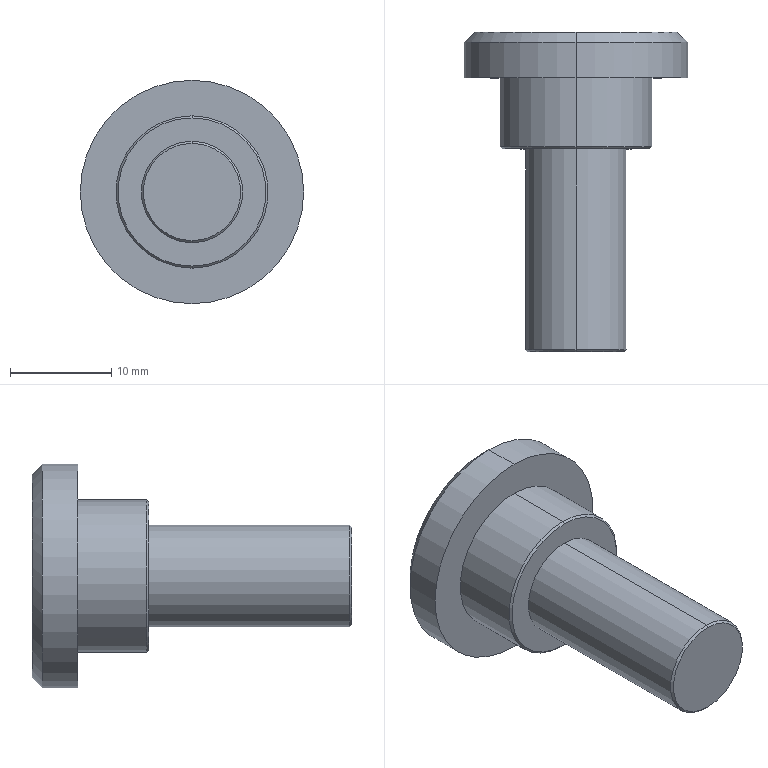Part | SolidWorks | features Chamfer 3, ICE 3, Extrusion 1 | 1 solid | 23 faces | box 22 x 31.5 x 22 mm | volume 4428 mm3 | plane 11 | cone 6 | cylinder 6 | commonest cylinder face diameters 10 x2 15 x2 22 x2
STEP:
#1=CARTESIAN_POINT('',(0.,0.,-4.8));
#2=VERTEX_POINT('',#1);
#3=CARTESIAN_POINT('',(0.,0.,4.8));
#4=VERTEX_POINT('',#3);
#5=CARTESIAN_POINT('',(0.,0.,0.));
#6=DIRECTION('',(0.,-1.,0.));
#7=DIRECTION('',(0.,0.,1.));
#8=AXIS2_PLACEMENT_3D('',#5,#6,#7);
#9=CIRCLE('',#8,4.8);
#10=EDGE_CURVE('',#2,#4,#9,.T.);
#11=ORIENTED_EDGE('',*,*,#10,.F.);
#12=CARTESIAN_POINT('',(0.,0.2,-5.));
#13=VERTEX_POINT('',#12);
#14=CARTESIAN_POINT('',(0.,0.2,-5.));
#15=DIRECTION('',(0.,0.7071,-0.7071));
#16=VECTOR('',#15,1000.);
#17=LINE('',#14,#16);
#18=EDGE_CURVE('',#2,#13,#17,.T.);
#19=ORIENTED_EDGE('',*,*,#18,.T.);
#20=CARTESIAN_POINT('',(0.,0.2,5.));
#21=VERTEX_POINT('',#20);
#22=CARTESIAN_POINT('',(0.,0.2,0.));
#23=DIRECTION('',(0.,1.,0.));
#24=DIRECTION('',(0.,0.,1.));
#25=AXIS2_PLACEMENT_3D('',#22,#23,#24);
#26=CIRCLE('',#25,5.);
#27=EDGE_CURVE('',#21,#13,#26,.T.);
#28=ORIENTED_EDGE('',*,*,#27,.F.);
#29=CARTESIAN_POINT('',(0.,0.2,5.));
#30=DIRECTION('',(0.,0.7071,0.7071));
#31=VECTOR('',#30,1000.);
#32=LINE('',#29,#31);
#33=EDGE_CURVE('',#4,#21,#32,.T.);
#34=ORIENTED_EDGE('',*,*,#33,.F.);
#35=EDGE_LOOP('',(#11,#19,#28,#34));
#36=FACE_OUTER_BOUND('',#35,.T.);
#37=CARTESIAN_POINT('',(0.,0.2,0.));
#38=DIRECTION('',(0.,1.,0.));
#39=DIRECTION('',(0.,0.,1.));
#40=AXIS2_PLACEMENT_3D('',#37,#38,#39);
#41=CONICAL_SURFACE('',#40,5.,0.7854);
#42=ADVANCED_FACE('',(#36),#41,.T.);
#43=CARTESIAN_POINT('',(0.,20.,-7.3));
#44=VERTEX_POINT('',#43);
#45=CARTESIAN_POINT('',(0.,20.,7.3));
#46=VERTEX_POINT('',#45);
#47=CARTESIAN_POINT('',(0.,20.,0.));
#48=DIRECTION('',(0.,-1.,0.));
#49=DIRECTION('',(0.,0.,1.));
#50=AXIS2_PLACEMENT_3D('',#47,#48,#49);
#51=CIRCLE('',#50,7.3);
#52=EDGE_CURVE('',#44,#46,#51,.T.);
#53=ORIENTED_EDGE('',*,*,#52,.F.);
#54=CARTESIAN_POINT('',(0.,20.2,-7.5));
#55=VERTEX_POINT('',#54);
#56=CARTESIAN_POINT('',(0.,20.2,-7.5));
#57=DIRECTION('',(0.,0.7071,-0.7071));
#58=VECTOR('',#57,1000.);
#59=LINE('',#56,#58);
#60=EDGE_CURVE('',#44,#55,#59,.T.);
#61=ORIENTED_EDGE('',*,*,#60,.T.);
#62=CARTESIAN_POINT('',(0.,20.2,7.5));
#63=VERTEX_POINT('',#62);
#64=CARTESIAN_POINT('',(0.,20.2,0.));
#65=DIRECTION('',(0.,1.,0.));
#66=DIRECTION('',(0.,0.,1.));
#67=AXIS2_PLACEMENT_3D('',#64,#65,#66);
#68=CIRCLE('',#67,7.5);
#69=EDGE_CURVE('',#63,#55,#68,.T.);
#70=ORIENTED_EDGE('',*,*,#69,.F.);
#71=CARTESIAN_POINT('',(0.,20.2,7.5));
#72=DIRECTION('',(0.,0.7071,0.7071));
#73=VECTOR('',#72,1000.);
#74=LINE('',#71,#73);
#75=EDGE_CURVE('',#46,#63,#74,.T.);
#76=ORIENTED_EDGE('',*,*,#75,.F.);
#77=EDGE_LOOP('',(#53,#61,#70,#76));
#78=FACE_OUTER_BOUND('',#77,.T.);
#79=CARTESIAN_POINT('',(0.,20.2,0.));
#80=DIRECTION('',(0.,1.,0.));
#81=DIRECTION('',(0.,0.,1.));
#82=AXIS2_PLACEMENT_3D('',#79,#80,#81);
#83=CONICAL_SURFACE('',#82,7.5,0.7854);
#84=ADVANCED_FACE('',(#78),#83,.T.);
#85=CARTESIAN_POINT('',(0.,31.5,10.));
#86=VERTEX_POINT('',#85);
#87=CARTESIAN_POINT('',(0.,31.5,-10.));
#88=VERTEX_POINT('',#87);
#89=CARTESIAN_POINT('',(0.,31.5,0.));
#90=DIRECTION('',(0.,1.,0.));
#91=DIRECTION('',(0.,0.,1.));
#92=AXIS2_PLACEMENT_3D('',#89,#90,#91);
#93=CIRCLE('',#92,10.);
#94=EDGE_CURVE('',#86,#88,#93,.T.);
#95=ORIENTED_EDGE('',*,*,#94,.F.);
#96=CARTESIAN_POINT('',(0.,30.5,11.));
#97=VERTEX_POINT('',#96);
#98=CARTESIAN_POINT('',(0.,31.5,10.));
#99=DIRECTION('',(0.,-0.7071,0.7071));
#100=VECTOR('',#99,1000.);
#101=LINE('',#98,#100);
#102=EDGE_CURVE('',#86,#97,#101,.T.);
#103=ORIENTED_EDGE('',*,*,#102,.T.);
#104=CARTESIAN_POINT('',(0.,30.5,-11.));
#105=VERTEX_POINT('',#104);
#106=CARTESIAN_POINT('',(0.,30.5,0.));
#107=DIRECTION('',(0.,-1.,0.));
#108=DIRECTION('',(0.,0.,1.));
#109=AXIS2_PLACEMENT_3D('',#106,#107,#108);
#110=CIRCLE('',#109,11.);
#111=EDGE_CURVE('',#105,#97,#110,.T.);
#112=ORIENTED_EDGE('',*,*,#111,.F.);
#113=CARTESIAN_POINT('',(0.,31.5,-10.));
#114=DIRECTION('',(0.,-0.7071,-0.7071));
#115=VECTOR('',#114,1000.);
#116=LINE('',#113,#115);
#117=EDGE_CURVE('',#88,#105,#116,.T.);
#118=ORIENTED_EDGE('',*,*,#117,.F.);
#119=EDGE_LOOP('',(#95,#103,#112,#118));
#120=FACE_OUTER_BOUND('',#119,.T.);
#121=CARTESIAN_POINT('',(0.,31.5,0.));
#122=DIRECTION('',(0.,-1.,0.));
#123=DIRECTION('',(0.,0.,-1.));
#124=AXIS2_PLACEMENT_3D('',#121,#122,#123);
#125=CONICAL_SURFACE('',#124,10.,0.7854);
#126=ADVANCED_FACE('',(#120),#125,.T.);
#127=ORIENTED_EDGE('',*,*,#111,.T.);
#128=CARTESIAN_POINT('',(0.,27.,11.));
#129=VERTEX_POINT('',#128);
#130=CARTESIAN_POINT('',(0.,31.5,11.));
#131=DIRECTION('',(0.,-1.,0.));
#132=VECTOR('',#131,1000.);
#133=LINE('',#130,#132);
#134=EDGE_CURVE('',#97,#129,#133,.T.);
#135=ORIENTED_EDGE('',*,*,#134,.T.);
#136=CARTESIAN_POINT('',(0.,27.,-11.));
#137=VERTEX_POINT('',#136);
#138=CARTESIAN_POINT('',(0.,27.,0.));
#139=DIRECTION('',(0.,1.,0.));
#140=DIRECTION('',(0.,0.,1.));
#141=AXIS2_PLACEMENT_3D('',#138,#139,#140);
#142=CIRCLE('',#141,11.);
#143=EDGE_CURVE('',#129,#137,#142,.T.);
#144=ORIENTED_EDGE('',*,*,#143,.T.);
#145=CARTESIAN_POINT('',(0.,31.5,-11.));
#146=DIRECTION('',(0.,-1.,0.));
#147=VECTOR('',#146,1000.);
#148=LINE('',#145,#147);
#149=EDGE_CURVE('',#105,#137,#148,.T.);
#150=ORIENTED_EDGE('',*,*,#149,.F.);
#151=EDGE_LOOP('',(#127,#135,#144,#150));
#152=FACE_OUTER_BOUND('',#151,.T.);
#153=CARTESIAN_POINT('',(0.,31.5,0.));
#154=DIRECTION('',(0.,-1.,0.));
#155=DIRECTION('',(0.,0.,-1.));
#156=AXIS2_PLACEMENT_3D('',#153,#154,#155);
#157=CYLINDRICAL_SURFACE('',#156,11.);
#158=ADVANCED_FACE('',(#152),#157,.T.);
#159=CARTESIAN_POINT('',(0.,27.,7.5));
#160=VERTEX_POINT('',#159);
#161=CARTESIAN_POINT('',(0.,27.,-7.5));
#162=VERTEX_POINT('',#161);
#163=CARTESIAN_POINT('',(0.,27.,0.));
#164=DIRECTION('',(0.,1.,0.));
#165=DIRECTION('',(0.,0.,1.));
#166=AXIS2_PLACEMENT_3D('',#163,#164,#165);
#167=CIRCLE('',#166,7.5);
#168=EDGE_CURVE('',#160,#162,#167,.T.);
#169=ORIENTED_EDGE('',*,*,#168,.F.);
#170=CARTESIAN_POINT('',(0.,27.,7.5));
#171=DIRECTION('',(0.,-1.,0.));
#172=VECTOR('',#171,1000.);
#173=LINE('',#170,#172);
#174=EDGE_CURVE('',#160,#63,#173,.T.);
#175=ORIENTED_EDGE('',*,*,#174,.T.);
#176=ORIENTED_EDGE('',*,*,#69,.T.);
#177=CARTESIAN_POINT('',(0.,27.,-7.5));
#178=DIRECTION('',(0.,-1.,0.));
#179=VECTOR('',#178,1000.);
#180=LINE('',#177,#179);
#181=EDGE_CURVE('',#162,#55,#180,.T.);
#182=ORIENTED_EDGE('',*,*,#181,.F.);
#183=EDGE_LOOP('',(#169,#175,#176,#182));
#184=FACE_OUTER_BOUND('',#183,.T.);
#185=CARTESIAN_POINT('',(0.,27.,0.));
#186=DIRECTION('',(0.,-1.,0.));
#187=DIRECTION('',(0.,0.,-1.));
#188=AXIS2_PLACEMENT_3D('',#185,#186,#187);
#189=CYLINDRICAL_SURFACE('',#188,7.5);
#190=ADVANCED_FACE('',(#184),#189,.T.);
#191=CARTESIAN_POINT('',(0.,20.,5.));
#192=VERTEX_POINT('',#191);
#193=CARTESIAN_POINT('',(0.,20.,-5.));
#194=VERTEX_POINT('',#193);
#195=CARTESIAN_POINT('',(0.,20.,0.));
#196=DIRECTION('',(0.,1.,0.));
#197=DIRECTION('',(0.,0.,1.));
#198=AXIS2_PLACEMENT_3D('',#195,#196,#197);
#199=CIRCLE('',#198,5.);
#200=EDGE_CURVE('',#192,#194,#199,.T.);
#201=ORIENTED_EDGE('',*,*,#200,.F.);
#202=CARTESIAN_POINT('',(0.,20.,5.));
#203=DIRECTION('',(0.,-1.,0.));
#204=VECTOR('',#203,1000.);
#205=LINE('',#202,#204);
#206=EDGE_CURVE('',#192,#21,#205,.T.);
#207=ORIENTED_EDGE('',*,*,#206,.T.);
#208=ORIENTED_EDGE('',*,*,#27,.T.);
#209=CARTESIAN_POINT('',(0.,20.,-5.));
#210=DIRECTION('',(0.,-1.,0.));
#211=VECTOR('',#210,1000.);
#212=LINE('',#209,#211);
#213=EDGE_CURVE('',#194,#13,#212,.T.);
#214=ORIENTED_EDGE('',*,*,#213,.F.);
#215=EDGE_LOOP('',(#201,#207,#208,#214));
#216=FACE_OUTER_BOUND('',#215,.T.);
#217=CARTESIAN_POINT('',(0.,20.,0.));
#218=DIRECTION('',(0.,-1.,0.));
#219=DIRECTION('',(0.,0.,-1.));
#220=AXIS2_PLACEMENT_3D('',#217,#218,#219);
#221=CYLINDRICAL_SURFACE('',#220,5.);
#222=ADVANCED_FACE('',(#216),#221,.T.);
#223=ORIENTED_EDGE('',*,*,#206,.F.);
#224=CARTESIAN_POINT('',(0.,20.,0.));
#225=DIRECTION('',(0.,1.,0.));
#226=DIRECTION('',(0.,0.,1.));
#227=AXIS2_PLACEMENT_3D('',#224,#225,#226);
#228=CIRCLE('',#227,5.);
#229=EDGE_CURVE('',#194,#192,#228,.T.);
#230=ORIENTED_EDGE('',*,*,#229,.F.);
#231=ORIENTED_EDGE('',*,*,#213,.T.);
#232=CARTESIAN_POINT('',(0.,0.2,0.));
#233=DIRECTION('',(0.,1.,0.));
#234=DIRECTION('',(0.,0.,1.));
#235=AXIS2_PLACEMENT_3D('',#232,#233,#234);
#236=CIRCLE('',#235,5.);
#237=EDGE_CURVE('',#13,#21,#236,.T.);
#238=ORIENTED_EDGE('',*,*,#237,.T.);
#239=EDGE_LOOP('',(#223,#230,#231,#238));
#240=FACE_OUTER_BOUND('',#239,.T.);
#241=CARTESIAN_POINT('',(0.,20.,0.));
#242=DIRECTION('',(0.,-1.,0.));
#243=DIRECTION('',(0.,0.,-1.));
#244=AXIS2_PLACEMENT_3D('',#241,#242,#243);
#245=CYLINDRICAL_SURFACE('',#244,5.);
#246=ADVANCED_FACE('',(#240),#245,.T.);
#247=CARTESIAN_POINT('',(0.,0.,0.));
#248=DIRECTION('',(0.,-1.,0.));
#249=DIRECTION('',(0.,0.,1.));
#250=AXIS2_PLACEMENT_3D('',#247,#248,#249);
#251=CIRCLE('',#250,4.8);
#252=EDGE_CURVE('',#4,#2,#251,.T.);
#253=ORIENTED_EDGE('',*,*,#252,.T.);
#254=ORIENTED_EDGE('',*,*,#10,.T.);
#255=EDGE_LOOP('',(#253,#254));
#256=FACE_OUTER_BOUND('',#255,.T.);
#257=CARTESIAN_POINT('',(0.,0.,0.));
#258=DIRECTION('',(0.,1.,0.));
#259=DIRECTION('',(0.,0.,1.));
#260=AXIS2_PLACEMENT_3D('',#257,#258,#259);
#261=PLANE('',#260);
#262=ADVANCED_FACE('',(#256),#261,.F.);
#263=CARTESIAN_POINT('',(0.,20.,0.));
#264=DIRECTION('',(0.,-1.,0.));
#265=DIRECTION('',(0.,0.,1.));
#266=AXIS2_PLACEMENT_3D('',#263,#264,#265);
#267=CIRCLE('',#266,7.3);
#268=EDGE_CURVE('',#46,#44,#267,.T.);
#269=ORIENTED_EDGE('',*,*,#268,.T.);
#270=ORIENTED_EDGE('',*,*,#52,.T.);
#271=EDGE_LOOP('',(#269,#270));
#272=FACE_OUTER_BOUND('',#271,.T.);
#273=ORIENTED_EDGE('',*,*,#229,.T.);
#274=ORIENTED_EDGE('',*,*,#200,.T.);
#275=EDGE_LOOP('',(#273,#274));
#276=FACE_BOUND('',#275,.T.);
#277=CARTESIAN_POINT('',(0.,20.,0.));
#278=DIRECTION('',(0.,1.,0.));
#279=DIRECTION('',(0.,0.,1.));
#280=AXIS2_PLACEMENT_3D('',#277,#278,#279);
#281=PLANE('',#280);
#282=ADVANCED_FACE('',(#272,#276),#281,.F.);
#283=ORIENTED_EDGE('',*,*,#174,.F.);
#284=CARTESIAN_POINT('',(0.,27.,0.));
#285=DIRECTION('',(0.,1.,0.));
#286=DIRECTION('',(0.,0.,1.));
#287=AXIS2_PLACEMENT_3D('',#284,#285,#286);
#288=CIRCLE('',#287,7.5);
#289=EDGE_CURVE('',#162,#160,#288,.T.);
#290=ORIENTED_EDGE('',*,*,#289,.F.);
#291=ORIENTED_EDGE('',*,*,#181,.T.);
#292=CARTESIAN_POINT('',(0.,20.2,0.));
#293=DIRECTION('',(0.,1.,0.));
#294=DIRECTION('',(0.,0.,1.));
#295=AXIS2_PLACEMENT_3D('',#292,#293,#294);
#296=CIRCLE('',#295,7.5);
#297=EDGE_CURVE('',#55,#63,#296,.T.);
#298=ORIENTED_EDGE('',*,*,#297,.T.);
#299=EDGE_LOOP('',(#283,#290,#291,#298));
#300=FACE_OUTER_BOUND('',#299,.T.);
#301=CARTESIAN_POINT('',(0.,27.,0.));
#302=DIRECTION('',(0.,-1.,0.));
#303=DIRECTION('',(0.,0.,-1.));
#304=AXIS2_PLACEMENT_3D('',#301,#302,#303);
#305=CYLINDRICAL_SURFACE('',#304,7.5);
#306=ADVANCED_FACE('',(#300),#305,.T.);
#307=CARTESIAN_POINT('',(0.,27.,0.));
#308=DIRECTION('',(0.,1.,0.));
#309=DIRECTION('',(0.,0.,1.));
#310=AXIS2_PLACEMENT_3D('',#307,#308,#309);
#311=CIRCLE('',#310,11.);
#312=EDGE_CURVE('',#137,#129,#311,.T.);
#313=ORIENTED_EDGE('',*,*,#312,.F.);
#314=ORIENTED_EDGE('',*,*,#143,.F.);
#315=EDGE_LOOP('',(#313,#314));
#316=FACE_OUTER_BOUND('',#315,.T.);
#317=ORIENTED_EDGE('',*,*,#289,.T.);
#318=ORIENTED_EDGE('',*,*,#168,.T.);
#319=EDGE_LOOP('',(#317,#318));
#320=FACE_BOUND('',#319,.T.);
#321=CARTESIAN_POINT('',(0.,27.,0.));
#322=DIRECTION('',(0.,1.,0.));
#323=DIRECTION('',(0.,0.,1.));
#324=AXIS2_PLACEMENT_3D('',#321,#322,#323);
#325=PLANE('',#324);
#326=ADVANCED_FACE('',(#316,#320),#325,.F.);
#327=ORIENTED_EDGE('',*,*,#134,.F.);
#328=CARTESIAN_POINT('',(0.,30.5,0.));
#329=DIRECTION('',(0.,-1.,0.));
#330=DIRECTION('',(0.,0.,1.));
#331=AXIS2_PLACEMENT_3D('',#328,#329,#330);
#332=CIRCLE('',#331,11.);
#333=EDGE_CURVE('',#97,#105,#332,.T.);
#334=ORIENTED_EDGE('',*,*,#333,.T.);
#335=ORIENTED_EDGE('',*,*,#149,.T.);
#336=ORIENTED_EDGE('',*,*,#312,.T.);
#337=EDGE_LOOP('',(#327,#334,#335,#336));
#338=FACE_OUTER_BOUND('',#337,.T.);
#339=CARTESIAN_POINT('',(0.,31.5,0.));
#340=DIRECTION('',(0.,-1.,0.));
#341=DIRECTION('',(0.,0.,-1.));
#342=AXIS2_PLACEMENT_3D('',#339,#340,#341);
#343=CYLINDRICAL_SURFACE('',#342,11.);
#344=ADVANCED_FACE('',(#338),#343,.T.);
#345=CARTESIAN_POINT('',(1.155,31.5,2.));
#346=VERTEX_POINT('',#345);
#347=CARTESIAN_POINT('',(2.309,31.5,0.));
#348=VERTEX_POINT('',#347);
#349=CARTESIAN_POINT('',(1.155,31.5,2.));
#350=DIRECTION('',(0.5,0.,-0.866));
#351=VECTOR('',#350,1000.);
#352=LINE('',#349,#351);
#353=EDGE_CURVE('',#346,#348,#352,.T.);
#354=ORIENTED_EDGE('',*,*,#353,.F.);
#355=CARTESIAN_POINT('',(-1.155,31.5,2.));
#356=VERTEX_POINT('',#355);
#357=CARTESIAN_POINT('',(-1.155,31.5,2.));
#358=DIRECTION('',(1.,0.,0.));
#359=VECTOR('',#358,1000.);
#360=LINE('',#357,#359);
#361=EDGE_CURVE('',#356,#346,#360,.T.);
#362=ORIENTED_EDGE('',*,*,#361,.F.);
#363=CARTESIAN_POINT('',(-2.309,31.5,0.));
#364=VERTEX_POINT('',#363);
#365=CARTESIAN_POINT('',(-2.309,31.5,0.));
#366=DIRECTION('',(0.5,0.,0.866));
#367=VECTOR('',#366,1000.);
#368=LINE('',#365,#367);
#369=EDGE_CURVE('',#364,#356,#368,.T.);
#370=ORIENTED_EDGE('',*,*,#369,.F.);
#371=CARTESIAN_POINT('',(-1.155,31.5,-2.));
#372=VERTEX_POINT('',#371);
#373=CARTESIAN_POINT('',(-1.155,31.5,-2.));
#374=DIRECTION('',(-0.5,0.,0.866));
#375=VECTOR('',#374,1000.);
#376=LINE('',#373,#375);
#377=EDGE_CURVE('',#372,#364,#376,.T.);
#378=ORIENTED_EDGE('',*,*,#377,.F.);
#379=CARTESIAN_POINT('',(1.155,31.5,-2.));
#380=VERTEX_POINT('',#379);
#381=CARTESIAN_POINT('',(1.155,31.5,-2.));
#382=DIRECTION('',(-1.,0.,0.));
#383=VECTOR('',#382,1000.);
#384=LINE('',#381,#383);
#385=EDGE_CURVE('',#380,#372,#384,.T.);
#386=ORIENTED_EDGE('',*,*,#385,.F.);
#387=CARTESIAN_POINT('',(2.309,31.5,0.));
#388=DIRECTION('',(-0.5,0.,-0.866));
#389=VECTOR('',#388,1000.);
#390=LINE('',#387,#389);
#391=EDGE_CURVE('',#348,#380,#390,.T.);
#392=ORIENTED_EDGE('',*,*,#391,.F.);
#393=EDGE_LOOP('',(#354,#362,#370,#378,#386,#392));
#394=FACE_BOUND('',#393,.T.);
#395=CARTESIAN_POINT('',(0.,31.5,0.));
#396=DIRECTION('',(0.,1.,0.));
#397=DIRECTION('',(0.,0.,1.));
#398=AXIS2_PLACEMENT_3D('',#395,#396,#397);
#399=CIRCLE('',#398,10.);
#400=EDGE_CURVE('',#88,#86,#399,.T.);
#401=ORIENTED_EDGE('',*,*,#400,.T.);
#402=ORIENTED_EDGE('',*,*,#94,.T.);
#403=EDGE_LOOP('',(#401,#402));
#404=FACE_OUTER_BOUND('',#403,.T.);
#405=CARTESIAN_POINT('',(0.,31.5,0.));
#406=DIRECTION('',(0.,1.,0.));
#407=DIRECTION('',(0.,0.,1.));
#408=AXIS2_PLACEMENT_3D('',#405,#406,#407);
#409=PLANE('',#408);
#410=ADVANCED_FACE('',(#394,#404),#409,.T.);
#411=ORIENTED_EDGE('',*,*,#102,.F.);
#412=ORIENTED_EDGE('',*,*,#400,.F.);
#413=ORIENTED_EDGE('',*,*,#117,.T.);
#414=ORIENTED_EDGE('',*,*,#333,.F.);
#415=EDGE_LOOP('',(#411,#412,#413,#414));
#416=FACE_OUTER_BOUND('',#415,.T.);
#417=CARTESIAN_POINT('',(0.,31.5,0.));
#418=DIRECTION('',(0.,-1.,0.));
#419=DIRECTION('',(0.,0.,-1.));
#420=AXIS2_PLACEMENT_3D('',#417,#418,#419);
#421=CONICAL_SURFACE('',#420,10.,0.7854);
#422=ADVANCED_FACE('',(#416),#421,.T.);
#423=ORIENTED_EDGE('',*,*,#60,.F.);
#424=ORIENTED_EDGE('',*,*,#268,.F.);
#425=ORIENTED_EDGE('',*,*,#75,.T.);
#426=ORIENTED_EDGE('',*,*,#297,.F.);
#427=EDGE_LOOP('',(#423,#424,#425,#426));
#428=FACE_OUTER_BOUND('',#427,.T.);
#429=CARTESIAN_POINT('',(0.,20.2,0.));
#430=DIRECTION('',(0.,1.,0.));
#431=DIRECTION('',(0.,0.,1.));
#432=AXIS2_PLACEMENT_3D('',#429,#430,#431);
#433=CONICAL_SURFACE('',#432,7.5,0.7854);
#434=ADVANCED_FACE('',(#428),#433,.T.);
#435=ORIENTED_EDGE('',*,*,#18,.F.);
#436=ORIENTED_EDGE('',*,*,#252,.F.);
#437=ORIENTED_EDGE('',*,*,#33,.T.);
#438=ORIENTED_EDGE('',*,*,#237,.F.);
#439=EDGE_LOOP('',(#435,#436,#437,#438));
#440=FACE_OUTER_BOUND('',#439,.T.);
#441=CARTESIAN_POINT('',(0.,0.2,0.));
#442=DIRECTION('',(0.,1.,0.));
#443=DIRECTION('',(0.,0.,1.));
#444=AXIS2_PLACEMENT_3D('',#441,#442,#443);
#445=CONICAL_SURFACE('',#444,5.,0.7854);
#446=ADVANCED_FACE('',(#440),#445,.T.);
#447=ORIENTED_EDGE('',*,*,#353,.T.);
#448=CARTESIAN_POINT('',(2.309,27.5,0.));
#449=VERTEX_POINT('',#448);
#450=CARTESIAN_POINT('',(2.309,27.5,0.));
#451=DIRECTION('',(0.,1.,0.));
#452=VECTOR('',#451,1000.);
#453=LINE('',#450,#452);
#454=EDGE_CURVE('',#449,#348,#453,.T.);
#455=ORIENTED_EDGE('',*,*,#454,.F.);
#456=CARTESIAN_POINT('',(1.155,27.5,2.));
#457=VERTEX_POINT('',#456);
#458=CARTESIAN_POINT('',(1.155,27.5,2.));
#459=DIRECTION('',(0.5,0.,-0.866));
#460=VECTOR('',#459,1000.);
#461=LINE('',#458,#460);
#462=EDGE_CURVE('',#457,#449,#461,.T.);
#463=ORIENTED_EDGE('',*,*,#462,.F.);
#464=CARTESIAN_POINT('',(1.155,27.5,2.));
#465=DIRECTION('',(0.,1.,0.));
#466=VECTOR('',#465,1000.);
#467=LINE('',#464,#466);
#468=EDGE_CURVE('',#457,#346,#467,.T.);
#469=ORIENTED_EDGE('',*,*,#468,.T.);
#470=EDGE_LOOP('',(#447,#455,#463,#469));
#471=FACE_OUTER_BOUND('',#470,.T.);
#472=CARTESIAN_POINT('',(1.155,27.5,2.));
#473=DIRECTION('',(0.866,0.,0.5));
#474=DIRECTION('',(0.5,0.,-0.866));
#475=AXIS2_PLACEMENT_3D('',#472,#473,#474);
#476=PLANE('',#475);
#477=ADVANCED_FACE('',(#471),#476,.F.);
#478=ORIENTED_EDGE('',*,*,#361,.T.);
#479=ORIENTED_EDGE('',*,*,#468,.F.);
#480=CARTESIAN_POINT('',(-1.155,27.5,2.));
#481=VERTEX_POINT('',#480);
#482=CARTESIAN_POINT('',(-1.155,27.5,2.));
#483=DIRECTION('',(1.,0.,0.));
#484=VECTOR('',#483,1000.);
#485=LINE('',#482,#484);
#486=EDGE_CURVE('',#481,#457,#485,.T.);
#487=ORIENTED_EDGE('',*,*,#486,.F.);
#488=CARTESIAN_POINT('',(-1.155,27.5,2.));
#489=DIRECTION('',(0.,1.,0.));
#490=VECTOR('',#489,1000.);
#491=LINE('',#488,#490);
#492=EDGE_CURVE('',#481,#356,#491,.T.);
#493=ORIENTED_EDGE('',*,*,#492,.T.);
#494=EDGE_LOOP('',(#478,#479,#487,#493));
#495=FACE_OUTER_BOUND('',#494,.T.);
#496=CARTESIAN_POINT('',(-1.155,27.5,2.));
#497=DIRECTION('',(0.,0.,1.));
#498=DIRECTION('',(1.,0.,0.));
#499=AXIS2_PLACEMENT_3D('',#496,#497,#498);
#500=PLANE('',#499);
#501=ADVANCED_FACE('',(#495),#500,.F.);
#502=ORIENTED_EDGE('',*,*,#369,.T.);
#503=ORIENTED_EDGE('',*,*,#492,.F.);
#504=CARTESIAN_POINT('',(-2.309,27.5,0.));
#505=VERTEX_POINT('',#504);
#506=CARTESIAN_POINT('',(-2.309,27.5,0.));
#507=DIRECTION('',(0.5,0.,0.866));
#508=VECTOR('',#507,1000.);
#509=LINE('',#506,#508);
#510=EDGE_CURVE('',#505,#481,#509,.T.);
#511=ORIENTED_EDGE('',*,*,#510,.F.);
#512=CARTESIAN_POINT('',(-2.309,27.5,0.));
#513=DIRECTION('',(0.,1.,0.));
#514=VECTOR('',#513,1000.);
#515=LINE('',#512,#514);
#516=EDGE_CURVE('',#505,#364,#515,.T.);
#517=ORIENTED_EDGE('',*,*,#516,.T.);
#518=EDGE_LOOP('',(#502,#503,#511,#517));
#519=FACE_OUTER_BOUND('',#518,.T.);
#520=CARTESIAN_POINT('',(-2.309,27.5,0.));
#521=DIRECTION('',(-0.866,0.,0.5));
#522=DIRECTION('',(0.5,0.,0.866));
#523=AXIS2_PLACEMENT_3D('',#520,#521,#522);
#524=PLANE('',#523);
#525=ADVANCED_FACE('',(#519),#524,.F.);
#526=ORIENTED_EDGE('',*,*,#377,.T.);
#527=ORIENTED_EDGE('',*,*,#516,.F.);
#528=CARTESIAN_POINT('',(-1.155,27.5,-2.));
#529=VERTEX_POINT('',#528);
#530=CARTESIAN_POINT('',(-1.155,27.5,-2.));
#531=DIRECTION('',(-0.5,0.,0.866));
#532=VECTOR('',#531,1000.);
#533=LINE('',#530,#532);
#534=EDGE_CURVE('',#529,#505,#533,.T.);
#535=ORIENTED_EDGE('',*,*,#534,.F.);
#536=CARTESIAN_POINT('',(-1.155,27.5,-2.));
#537=DIRECTION('',(0.,1.,0.));
#538=VECTOR('',#537,1000.);
#539=LINE('',#536,#538);
#540=EDGE_CURVE('',#529,#372,#539,.T.);
#541=ORIENTED_EDGE('',*,*,#540,.T.);
#542=EDGE_LOOP('',(#526,#527,#535,#541));
#543=FACE_OUTER_BOUND('',#542,.T.);
#544=CARTESIAN_POINT('',(-1.155,27.5,-2.));
#545=DIRECTION('',(-0.866,0.,-0.5));
#546=DIRECTION('',(-0.5,0.,0.866));
#547=AXIS2_PLACEMENT_3D('',#544,#545,#546);
#548=PLANE('',#547);
#549=ADVANCED_FACE('',(#543),#548,.F.);
#550=ORIENTED_EDGE('',*,*,#385,.T.);
#551=ORIENTED_EDGE('',*,*,#540,.F.);
#552=CARTESIAN_POINT('',(1.155,27.5,-2.));
#553=VERTEX_POINT('',#552);
#554=CARTESIAN_POINT('',(1.155,27.5,-2.));
#555=DIRECTION('',(-1.,0.,0.));
#556=VECTOR('',#555,1000.);
#557=LINE('',#554,#556);
#558=EDGE_CURVE('',#553,#529,#557,.T.);
#559=ORIENTED_EDGE('',*,*,#558,.F.);
#560=CARTESIAN_POINT('',(1.155,27.5,-2.));
#561=DIRECTION('',(0.,1.,0.));
#562=VECTOR('',#561,1000.);
#563=LINE('',#560,#562);
#564=EDGE_CURVE('',#553,#380,#563,.T.);
#565=ORIENTED_EDGE('',*,*,#564,.T.);
#566=EDGE_LOOP('',(#550,#551,#559,#565));
#567=FACE_OUTER_BOUND('',#566,.T.);
#568=CARTESIAN_POINT('',(1.155,27.5,-2.));
#569=DIRECTION('',(0.,0.,-1.));
#570=DIRECTION('',(-1.,0.,0.));
#571=AXIS2_PLACEMENT_3D('',#568,#569,#570);
#572=PLANE('',#571);
#573=ADVANCED_FACE('',(#567),#572,.F.);
#574=ORIENTED_EDGE('',*,*,#391,.T.);
#575=ORIENTED_EDGE('',*,*,#564,.F.);
#576=CARTESIAN_POINT('',(2.309,27.5,0.));
#577=DIRECTION('',(-0.5,0.,-0.866));
#578=VECTOR('',#577,1000.);
#579=LINE('',#576,#578);
#580=EDGE_CURVE('',#449,#553,#579,.T.);
#581=ORIENTED_EDGE('',*,*,#580,.F.);
#582=ORIENTED_EDGE('',*,*,#454,.T.);
#583=EDGE_LOOP('',(#574,#575,#581,#582));
#584=FACE_OUTER_BOUND('',#583,.T.);
#585=CARTESIAN_POINT('',(2.309,27.5,0.));
#586=DIRECTION('',(0.866,0.,-0.5));
#587=DIRECTION('',(-0.5,0.,-0.866));
#588=AXIS2_PLACEMENT_3D('',#585,#586,#587);
#589=PLANE('',#588);
#590=ADVANCED_FACE('',(#584),#589,.F.);
#591=ORIENTED_EDGE('',*,*,#462,.T.);
#592=ORIENTED_EDGE('',*,*,#580,.T.);
#593=ORIENTED_EDGE('',*,*,#558,.T.);
#594=ORIENTED_EDGE('',*,*,#534,.T.);
#595=ORIENTED_EDGE('',*,*,#510,.T.);
#596=ORIENTED_EDGE('',*,*,#486,.T.);
#597=EDGE_LOOP('',(#591,#592,#593,#594,#595,#596));
#598=FACE_OUTER_BOUND('',#597,.T.);
#599=CARTESIAN_POINT('',(0.,27.5,0.));
#600=DIRECTION('',(0.,1.,0.));
#601=DIRECTION('',(0.,0.,1.));
#602=AXIS2_PLACEMENT_3D('',#599,#600,#601);
#603=PLANE('',#602);
#604=ADVANCED_FACE('',(#598),#603,.T.);
#605=CLOSED_SHELL('',(#42,#84,#126,#158,#190,#222,#246,#262,#282,#306,#326,#344,#410,#422,#434,#446,#477,#501,#525,#549,#573,#590,#604));
#606=MANIFOLD_SOLID_BREP('',#605);
#607=CARTESIAN_POINT('',(0.,0.,0.));
#608=DIRECTION('',(0.,0.,1.));
#609=DIRECTION('',(1.,0.,0.));
#610=AXIS2_PLACEMENT_3D('',#607,#608,#609);
#611=(LENGTH_UNIT()NAMED_UNIT(*)SI_UNIT(.MILLI.,.METRE.));
#612=UNCERTAINTY_MEASURE_WITH_UNIT(LENGTH_MEASURE(0.00001),#611,'','');
#613=(NAMED_UNIT(*)PLANE_ANGLE_UNIT()SI_UNIT($,.RADIAN.));
#614=(NAMED_UNIT(*)SI_UNIT($,.STERADIAN.)SOLID_ANGLE_UNIT());
#615=(GEOMETRIC_REPRESENTATION_CONTEXT(3)GLOBAL_UNCERTAINTY_ASSIGNED_CONTEXT((#612))GLOBAL_UNIT_ASSIGNED_CONTEXT((#611,#613,#614))REPRESENTATION_CONTEXT('',''));
#616=ADVANCED_BREP_SHAPE_REPRESENTATION('',(#606,#610),#615);